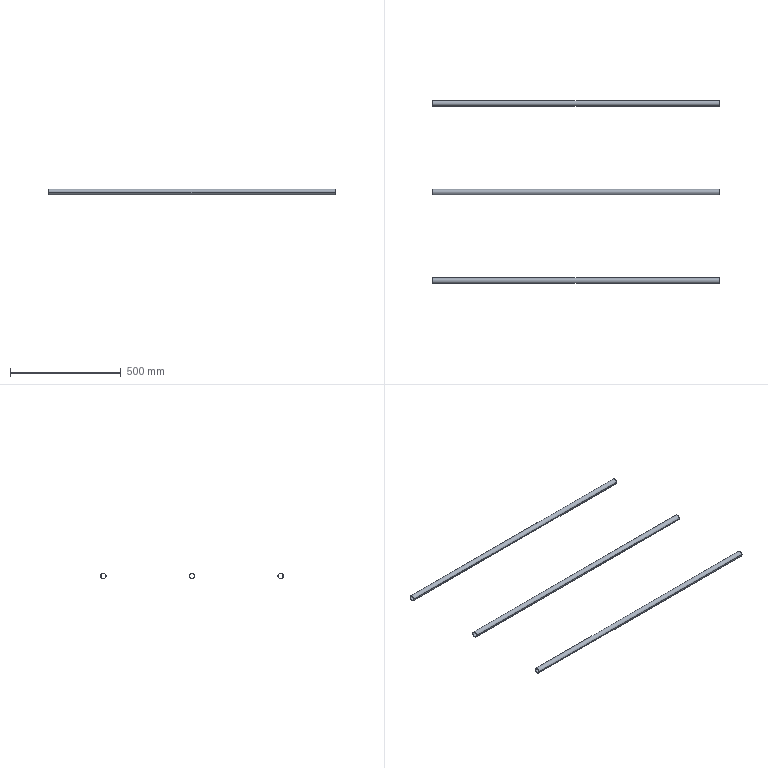Part | STEP file | E3-中转釜护栏6栏杆_Default<As Machined> | 3 solids | 18 faces | box 1295 x 825 x 25 mm | volume 430229 mm3 | cylinder 12 | plane 6 | commonest cylinder face diameters 22 x6 25 x6
STEP:
#1=CARTESIAN_POINT('',(0.,0.,0.));
#2=DIRECTION('',(0.,0.,1.));
#3=DIRECTION('',(1.,0.,0.));
#4=AXIS2_PLACEMENT_3D('',#1,#2,#3);
#5=CARTESIAN_POINT('',(647.5,787.5,0.));
#6=VERTEX_POINT('',#5);
#7=CARTESIAN_POINT('',(647.5,812.5,0.));
#8=VERTEX_POINT('',#7);
#9=CARTESIAN_POINT('',(647.5,800.,0.));
#10=DIRECTION('',(-1.,0.,0.));
#11=DIRECTION('',(0.,1.,0.));
#12=AXIS2_PLACEMENT_3D('',#9,#10,#11);
#13=CIRCLE('',#12,12.5);
#14=CARTESIAN_POINT('',(647.5,800.,0.));
#15=DIRECTION('',(-1.,0.,0.));
#16=DIRECTION('',(0.,-1.,0.));
#17=AXIS2_PLACEMENT_3D('',#14,#15,#16);
#18=CYLINDRICAL_SURFACE('',#17,12.5);
#19=CARTESIAN_POINT('',(-3.142,0.));
#20=DIRECTION('',(1.,0.));
#21=VECTOR('',#20,1.);
#22=LINE('',#19,#21);
#23=(GEOMETRIC_REPRESENTATION_CONTEXT(2)PARAMETRIC_REPRESENTATION_CONTEXT()REPRESENTATION_CONTEXT('',''));
#24=DEFINITIONAL_REPRESENTATION('',(#22),#23);
#25=PCURVE('',#18,#24);
#26=CARTESIAN_POINT('',(647.5,800.,0.));
#27=DIRECTION('',(1.,0.,0.));
#28=DIRECTION('',(0.,1.,0.));
#29=AXIS2_PLACEMENT_3D('',#26,#27,#28);
#30=PLANE('',#29);
#31=CARTESIAN_POINT('',(12.5,0.));
#32=CARTESIAN_POINT('',(12.5,-21.651));
#33=CARTESIAN_POINT('',(-6.25,-10.825));
#34=CARTESIAN_POINT('',(-25.,0.));
#35=CARTESIAN_POINT('',(-6.25,10.825));
#36=CARTESIAN_POINT('',(12.5,21.651));
#37=CARTESIAN_POINT('',(12.5,0.));
#38=(BOUNDED_CURVE()B_SPLINE_CURVE(2,(#31,#32,#33,#34,#35,#36,#37),.UNSPECIFIED.,.T.,.F.)B_SPLINE_CURVE_WITH_KNOTS((1,2,2,2,2,1),(-2.094,0.,2.094,4.189,6.283,8.378),.UNSPECIFIED.)CURVE()GEOMETRIC_REPRESENTATION_ITEM()RATIONAL_B_SPLINE_CURVE((1.,0.5,1.,0.5,1.,0.5,1.))REPRESENTATION_ITEM(''));
#39=(GEOMETRIC_REPRESENTATION_CONTEXT(2)PARAMETRIC_REPRESENTATION_CONTEXT()REPRESENTATION_CONTEXT('',''));
#40=DEFINITIONAL_REPRESENTATION('',(#38),#39);
#41=PCURVE('',#30,#40);
#42=SURFACE_CURVE('',#13,(#25,#41),.PCURVE_S1.);
#43=EDGE_CURVE('',#6,#8,#42,.T.);
#44=ORIENTED_EDGE('',*,*,#43,.T.);
#45=CARTESIAN_POINT('',(-647.5,812.5,0.));
#46=VERTEX_POINT('',#45);
#47=CARTESIAN_POINT('',(647.5,812.5,0.));
#48=DIRECTION('',(-1.,0.,0.));
#49=VECTOR('',#48,1.);
#50=LINE('',#47,#49);
#51=CARTESIAN_POINT('',(3.142,0.));
#52=DIRECTION('',(0.,1.));
#53=VECTOR('',#52,1.);
#54=LINE('',#51,#53);
#55=(GEOMETRIC_REPRESENTATION_CONTEXT(2)PARAMETRIC_REPRESENTATION_CONTEXT()REPRESENTATION_CONTEXT('',''));
#56=DEFINITIONAL_REPRESENTATION('',(#54),#55);
#57=PCURVE('',#18,#56);
#58=CARTESIAN_POINT('',(647.5,800.,0.));
#59=DIRECTION('',(-1.,0.,0.));
#60=DIRECTION('',(0.,-1.,0.));
#61=AXIS2_PLACEMENT_3D('',#58,#59,#60);
#62=CYLINDRICAL_SURFACE('',#61,12.5);
#63=CARTESIAN_POINT('',(3.142,0.));
#64=DIRECTION('',(0.,1.));
#65=VECTOR('',#64,1.);
#66=LINE('',#63,#65);
#67=(GEOMETRIC_REPRESENTATION_CONTEXT(2)PARAMETRIC_REPRESENTATION_CONTEXT()REPRESENTATION_CONTEXT('',''));
#68=DEFINITIONAL_REPRESENTATION('',(#66),#67);
#69=PCURVE('',#62,#68);
#70=SURFACE_CURVE('',#50,(#57,#69),.PCURVE_S1.);
#71=EDGE_CURVE('',#8,#46,#70,.T.);
#72=ORIENTED_EDGE('',*,*,#71,.T.);
#73=CARTESIAN_POINT('',(-647.5,787.5,0.));
#74=VERTEX_POINT('',#73);
#75=CARTESIAN_POINT('',(-647.5,800.,0.));
#76=DIRECTION('',(-1.,0.,0.));
#77=DIRECTION('',(0.,1.,0.));
#78=AXIS2_PLACEMENT_3D('',#75,#76,#77);
#79=CIRCLE('',#78,12.5);
#80=CARTESIAN_POINT('',(-3.142,1295.));
#81=DIRECTION('',(1.,0.));
#82=VECTOR('',#81,1.);
#83=LINE('',#80,#82);
#84=(GEOMETRIC_REPRESENTATION_CONTEXT(2)PARAMETRIC_REPRESENTATION_CONTEXT()REPRESENTATION_CONTEXT('',''));
#85=DEFINITIONAL_REPRESENTATION('',(#83),#84);
#86=PCURVE('',#18,#85);
#87=CARTESIAN_POINT('',(-647.5,800.,0.));
#88=DIRECTION('',(1.,0.,0.));
#89=DIRECTION('',(0.,1.,0.));
#90=AXIS2_PLACEMENT_3D('',#87,#88,#89);
#91=PLANE('',#90);
#92=CARTESIAN_POINT('',(12.5,0.));
#93=CARTESIAN_POINT('',(12.5,-21.651));
#94=CARTESIAN_POINT('',(-6.25,-10.825));
#95=CARTESIAN_POINT('',(-25.,0.));
#96=CARTESIAN_POINT('',(-6.25,10.825));
#97=CARTESIAN_POINT('',(12.5,21.651));
#98=CARTESIAN_POINT('',(12.5,0.));
#99=(BOUNDED_CURVE()B_SPLINE_CURVE(2,(#92,#93,#94,#95,#96,#97,#98),.UNSPECIFIED.,.T.,.F.)B_SPLINE_CURVE_WITH_KNOTS((1,2,2,2,2,1),(-2.094,0.,2.094,4.189,6.283,8.378),.UNSPECIFIED.)CURVE()GEOMETRIC_REPRESENTATION_ITEM()RATIONAL_B_SPLINE_CURVE((1.,0.5,1.,0.5,1.,0.5,1.))REPRESENTATION_ITEM(''));
#100=(GEOMETRIC_REPRESENTATION_CONTEXT(2)PARAMETRIC_REPRESENTATION_CONTEXT()REPRESENTATION_CONTEXT('',''));
#101=DEFINITIONAL_REPRESENTATION('',(#99),#100);
#102=PCURVE('',#91,#101);
#103=SURFACE_CURVE('',#79,(#86,#102),.PCURVE_S1.);
#104=EDGE_CURVE('',#74,#46,#103,.T.);
#105=ORIENTED_EDGE('',*,*,#104,.F.);
#106=CARTESIAN_POINT('',(647.5,787.5,0.));
#107=DIRECTION('',(-1.,0.,0.));
#108=VECTOR('',#107,1.);
#109=LINE('',#106,#108);
#110=CARTESIAN_POINT('',(0.,0.));
#111=DIRECTION('',(0.,1.));
#112=VECTOR('',#111,1.);
#113=LINE('',#110,#112);
#114=(GEOMETRIC_REPRESENTATION_CONTEXT(2)PARAMETRIC_REPRESENTATION_CONTEXT()REPRESENTATION_CONTEXT('',''));
#115=DEFINITIONAL_REPRESENTATION('',(#113),#114);
#116=PCURVE('',#18,#115);
#117=CARTESIAN_POINT('',(6.283,0.));
#118=DIRECTION('',(0.,1.));
#119=VECTOR('',#118,1.);
#120=LINE('',#117,#119);
#121=(GEOMETRIC_REPRESENTATION_CONTEXT(2)PARAMETRIC_REPRESENTATION_CONTEXT()REPRESENTATION_CONTEXT('',''));
#122=DEFINITIONAL_REPRESENTATION('',(#120),#121);
#123=PCURVE('',#62,#122);
#124=SURFACE_CURVE('',#109,(#116,#123),.PCURVE_S1.);
#125=EDGE_CURVE('',#6,#74,#124,.T.);
#126=ORIENTED_EDGE('',*,*,#125,.F.);
#127=EDGE_LOOP('',(#44,#72,#105,#126));
#128=FACE_BOUND('',#127,.T.);
#129=ADVANCED_FACE('',(#128),#18,.T.);
#130=CARTESIAN_POINT('',(647.5,789.,0.));
#131=VERTEX_POINT('',#130);
#132=CARTESIAN_POINT('',(-647.5,789.,0.));
#133=VERTEX_POINT('',#132);
#134=CARTESIAN_POINT('',(647.5,789.,0.));
#135=DIRECTION('',(-1.,0.,0.));
#136=VECTOR('',#135,1.);
#137=LINE('',#134,#136);
#138=CARTESIAN_POINT('',(647.5,800.,0.));
#139=DIRECTION('',(-1.,0.,0.));
#140=DIRECTION('',(0.,-1.,0.));
#141=AXIS2_PLACEMENT_3D('',#138,#139,#140);
#142=CYLINDRICAL_SURFACE('',#141,11.);
#143=CARTESIAN_POINT('',(6.283,0.));
#144=DIRECTION('',(0.,1.));
#145=VECTOR('',#144,1.);
#146=LINE('',#143,#145);
#147=(GEOMETRIC_REPRESENTATION_CONTEXT(2)PARAMETRIC_REPRESENTATION_CONTEXT()REPRESENTATION_CONTEXT('',''));
#148=DEFINITIONAL_REPRESENTATION('',(#146),#147);
#149=PCURVE('',#142,#148);
#150=CARTESIAN_POINT('',(647.5,800.,0.));
#151=DIRECTION('',(-1.,0.,0.));
#152=DIRECTION('',(0.,-1.,0.));
#153=AXIS2_PLACEMENT_3D('',#150,#151,#152);
#154=CYLINDRICAL_SURFACE('',#153,11.);
#155=CARTESIAN_POINT('',(0.,0.));
#156=DIRECTION('',(0.,1.));
#157=VECTOR('',#156,1.);
#158=LINE('',#155,#157);
#159=(GEOMETRIC_REPRESENTATION_CONTEXT(2)PARAMETRIC_REPRESENTATION_CONTEXT()REPRESENTATION_CONTEXT('',''));
#160=DEFINITIONAL_REPRESENTATION('',(#158),#159);
#161=PCURVE('',#154,#160);
#162=SURFACE_CURVE('',#137,(#149,#161),.PCURVE_S1.);
#163=EDGE_CURVE('',#131,#133,#162,.T.);
#164=ORIENTED_EDGE('',*,*,#163,.T.);
#165=CARTESIAN_POINT('',(-647.5,811.,0.));
#166=VERTEX_POINT('',#165);
#167=CARTESIAN_POINT('',(-647.5,800.,0.));
#168=DIRECTION('',(-1.,0.,0.));
#169=DIRECTION('',(0.,1.,0.));
#170=AXIS2_PLACEMENT_3D('',#167,#168,#169);
#171=CIRCLE('',#170,11.);
#172=CARTESIAN_POINT('',(3.142,1295.));
#173=DIRECTION('',(1.,0.));
#174=VECTOR('',#173,1.);
#175=LINE('',#172,#174);
#176=(GEOMETRIC_REPRESENTATION_CONTEXT(2)PARAMETRIC_REPRESENTATION_CONTEXT()REPRESENTATION_CONTEXT('',''));
#177=DEFINITIONAL_REPRESENTATION('',(#175),#176);
#178=PCURVE('',#142,#177);
#179=CARTESIAN_POINT('',(11.,0.));
#180=CARTESIAN_POINT('',(11.,-19.053));
#181=CARTESIAN_POINT('',(-5.5,-9.526));
#182=CARTESIAN_POINT('',(-22.,0.));
#183=CARTESIAN_POINT('',(-5.5,9.526));
#184=CARTESIAN_POINT('',(11.,19.053));
#185=CARTESIAN_POINT('',(11.,0.));
#186=(BOUNDED_CURVE()B_SPLINE_CURVE(2,(#179,#180,#181,#182,#183,#184,#185),.UNSPECIFIED.,.T.,.F.)B_SPLINE_CURVE_WITH_KNOTS((1,2,2,2,2,1),(-2.094,0.,2.094,4.189,6.283,8.378),.UNSPECIFIED.)CURVE()GEOMETRIC_REPRESENTATION_ITEM()RATIONAL_B_SPLINE_CURVE((1.,0.5,1.,0.5,1.,0.5,1.))REPRESENTATION_ITEM(''));
#187=(GEOMETRIC_REPRESENTATION_CONTEXT(2)PARAMETRIC_REPRESENTATION_CONTEXT()REPRESENTATION_CONTEXT('',''));
#188=DEFINITIONAL_REPRESENTATION('',(#186),#187);
#189=PCURVE('',#91,#188);
#190=SURFACE_CURVE('',#171,(#178,#189),.PCURVE_S1.);
#191=EDGE_CURVE('',#166,#133,#190,.T.);
#192=ORIENTED_EDGE('',*,*,#191,.F.);
#193=CARTESIAN_POINT('',(647.5,811.,0.));
#194=VERTEX_POINT('',#193);
#195=CARTESIAN_POINT('',(647.5,811.,0.));
#196=DIRECTION('',(-1.,0.,0.));
#197=VECTOR('',#196,1.);
#198=LINE('',#195,#197);
#199=CARTESIAN_POINT('',(3.142,0.));
#200=DIRECTION('',(0.,1.));
#201=VECTOR('',#200,1.);
#202=LINE('',#199,#201);
#203=(GEOMETRIC_REPRESENTATION_CONTEXT(2)PARAMETRIC_REPRESENTATION_CONTEXT()REPRESENTATION_CONTEXT('',''));
#204=DEFINITIONAL_REPRESENTATION('',(#202),#203);
#205=PCURVE('',#142,#204);
#206=CARTESIAN_POINT('',(3.142,0.));
#207=DIRECTION('',(0.,1.));
#208=VECTOR('',#207,1.);
#209=LINE('',#206,#208);
#210=(GEOMETRIC_REPRESENTATION_CONTEXT(2)PARAMETRIC_REPRESENTATION_CONTEXT()REPRESENTATION_CONTEXT('',''));
#211=DEFINITIONAL_REPRESENTATION('',(#209),#210);
#212=PCURVE('',#154,#211);
#213=SURFACE_CURVE('',#198,(#205,#212),.PCURVE_S1.);
#214=EDGE_CURVE('',#194,#166,#213,.T.);
#215=ORIENTED_EDGE('',*,*,#214,.F.);
#216=CARTESIAN_POINT('',(647.5,800.,0.));
#217=DIRECTION('',(-1.,0.,0.));
#218=DIRECTION('',(0.,1.,0.));
#219=AXIS2_PLACEMENT_3D('',#216,#217,#218);
#220=CIRCLE('',#219,11.);
#221=CARTESIAN_POINT('',(3.142,0.));
#222=DIRECTION('',(1.,0.));
#223=VECTOR('',#222,1.);
#224=LINE('',#221,#223);
#225=(GEOMETRIC_REPRESENTATION_CONTEXT(2)PARAMETRIC_REPRESENTATION_CONTEXT()REPRESENTATION_CONTEXT('',''));
#226=DEFINITIONAL_REPRESENTATION('',(#224),#225);
#227=PCURVE('',#142,#226);
#228=CARTESIAN_POINT('',(11.,0.));
#229=CARTESIAN_POINT('',(11.,-19.053));
#230=CARTESIAN_POINT('',(-5.5,-9.526));
#231=CARTESIAN_POINT('',(-22.,0.));
#232=CARTESIAN_POINT('',(-5.5,9.526));
#233=CARTESIAN_POINT('',(11.,19.053));
#234=CARTESIAN_POINT('',(11.,0.));
#235=(BOUNDED_CURVE()B_SPLINE_CURVE(2,(#228,#229,#230,#231,#232,#233,#234),.UNSPECIFIED.,.T.,.F.)B_SPLINE_CURVE_WITH_KNOTS((1,2,2,2,2,1),(-2.094,0.,2.094,4.189,6.283,8.378),.UNSPECIFIED.)CURVE()GEOMETRIC_REPRESENTATION_ITEM()RATIONAL_B_SPLINE_CURVE((1.,0.5,1.,0.5,1.,0.5,1.))REPRESENTATION_ITEM(''));
#236=(GEOMETRIC_REPRESENTATION_CONTEXT(2)PARAMETRIC_REPRESENTATION_CONTEXT()REPRESENTATION_CONTEXT('',''));
#237=DEFINITIONAL_REPRESENTATION('',(#235),#236);
#238=PCURVE('',#30,#237);
#239=SURFACE_CURVE('',#220,(#227,#238),.PCURVE_S1.);
#240=EDGE_CURVE('',#194,#131,#239,.T.);
#241=ORIENTED_EDGE('',*,*,#240,.T.);
#242=EDGE_LOOP('',(#164,#192,#215,#241));
#243=FACE_BOUND('',#242,.F.);
#244=ADVANCED_FACE('',(#243),#142,.F.);
#245=CARTESIAN_POINT('',(-647.5,800.,0.));
#246=DIRECTION('',(-1.,0.,0.));
#247=DIRECTION('',(0.,1.,0.));
#248=AXIS2_PLACEMENT_3D('',#245,#246,#247);
#249=CIRCLE('',#248,11.);
#250=CARTESIAN_POINT('',(-3.142,1295.));
#251=DIRECTION('',(1.,0.));
#252=VECTOR('',#251,1.);
#253=LINE('',#250,#252);
#254=(GEOMETRIC_REPRESENTATION_CONTEXT(2)PARAMETRIC_REPRESENTATION_CONTEXT()REPRESENTATION_CONTEXT('',''));
#255=DEFINITIONAL_REPRESENTATION('',(#253),#254);
#256=PCURVE('',#154,#255);
#257=CARTESIAN_POINT('',(11.,0.));
#258=CARTESIAN_POINT('',(11.,-19.053));
#259=CARTESIAN_POINT('',(-5.5,-9.526));
#260=CARTESIAN_POINT('',(-22.,0.));
#261=CARTESIAN_POINT('',(-5.5,9.526));
#262=CARTESIAN_POINT('',(11.,19.053));
#263=CARTESIAN_POINT('',(11.,0.));
#264=(BOUNDED_CURVE()B_SPLINE_CURVE(2,(#257,#258,#259,#260,#261,#262,#263),.UNSPECIFIED.,.T.,.F.)B_SPLINE_CURVE_WITH_KNOTS((1,2,2,2,2,1),(-2.094,0.,2.094,4.189,6.283,8.378),.UNSPECIFIED.)CURVE()GEOMETRIC_REPRESENTATION_ITEM()RATIONAL_B_SPLINE_CURVE((1.,0.5,1.,0.5,1.,0.5,1.))REPRESENTATION_ITEM(''));
#265=(GEOMETRIC_REPRESENTATION_CONTEXT(2)PARAMETRIC_REPRESENTATION_CONTEXT()REPRESENTATION_CONTEXT('',''));
#266=DEFINITIONAL_REPRESENTATION('',(#264),#265);
#267=PCURVE('',#91,#266);
#268=SURFACE_CURVE('',#249,(#256,#267),.PCURVE_S1.);
#269=EDGE_CURVE('',#133,#166,#268,.T.);
#270=ORIENTED_EDGE('',*,*,#269,.F.);
#271=ORIENTED_EDGE('',*,*,#163,.F.);
#272=CARTESIAN_POINT('',(647.5,800.,0.));
#273=DIRECTION('',(-1.,0.,0.));
#274=DIRECTION('',(0.,1.,0.));
#275=AXIS2_PLACEMENT_3D('',#272,#273,#274);
#276=CIRCLE('',#275,11.);
#277=CARTESIAN_POINT('',(-3.142,0.));
#278=DIRECTION('',(1.,0.));
#279=VECTOR('',#278,1.);
#280=LINE('',#277,#279);
#281=(GEOMETRIC_REPRESENTATION_CONTEXT(2)PARAMETRIC_REPRESENTATION_CONTEXT()REPRESENTATION_CONTEXT('',''));
#282=DEFINITIONAL_REPRESENTATION('',(#280),#281);
#283=PCURVE('',#154,#282);
#284=CARTESIAN_POINT('',(11.,0.));
#285=CARTESIAN_POINT('',(11.,-19.053));
#286=CARTESIAN_POINT('',(-5.5,-9.526));
#287=CARTESIAN_POINT('',(-22.,0.));
#288=CARTESIAN_POINT('',(-5.5,9.526));
#289=CARTESIAN_POINT('',(11.,19.053));
#290=CARTESIAN_POINT('',(11.,0.));
#291=(BOUNDED_CURVE()B_SPLINE_CURVE(2,(#284,#285,#286,#287,#288,#289,#290),.UNSPECIFIED.,.T.,.F.)B_SPLINE_CURVE_WITH_KNOTS((1,2,2,2,2,1),(-2.094,0.,2.094,4.189,6.283,8.378),.UNSPECIFIED.)CURVE()GEOMETRIC_REPRESENTATION_ITEM()RATIONAL_B_SPLINE_CURVE((1.,0.5,1.,0.5,1.,0.5,1.))REPRESENTATION_ITEM(''));
#292=(GEOMETRIC_REPRESENTATION_CONTEXT(2)PARAMETRIC_REPRESENTATION_CONTEXT()REPRESENTATION_CONTEXT('',''));
#293=DEFINITIONAL_REPRESENTATION('',(#291),#292);
#294=PCURVE('',#30,#293);
#295=SURFACE_CURVE('',#276,(#283,#294),.PCURVE_S1.);
#296=EDGE_CURVE('',#131,#194,#295,.T.);
#297=ORIENTED_EDGE('',*,*,#296,.T.);
#298=ORIENTED_EDGE('',*,*,#214,.T.);
#299=EDGE_LOOP('',(#270,#271,#297,#298));
#300=FACE_BOUND('',#299,.F.);
#301=ADVANCED_FACE('',(#300),#154,.F.);
#302=ORIENTED_EDGE('',*,*,#71,.F.);
#303=CARTESIAN_POINT('',(647.5,800.,0.));
#304=DIRECTION('',(-1.,0.,0.));
#305=DIRECTION('',(0.,1.,0.));
#306=AXIS2_PLACEMENT_3D('',#303,#304,#305);
#307=CIRCLE('',#306,12.5);
#308=CARTESIAN_POINT('',(3.142,0.));
#309=DIRECTION('',(1.,0.));
#310=VECTOR('',#309,1.);
#311=LINE('',#308,#310);
#312=(GEOMETRIC_REPRESENTATION_CONTEXT(2)PARAMETRIC_REPRESENTATION_CONTEXT()REPRESENTATION_CONTEXT('',''));
#313=DEFINITIONAL_REPRESENTATION('',(#311),#312);
#314=PCURVE('',#62,#313);
#315=CARTESIAN_POINT('',(12.5,0.));
#316=CARTESIAN_POINT('',(12.5,-21.651));
#317=CARTESIAN_POINT('',(-6.25,-10.825));
#318=CARTESIAN_POINT('',(-25.,0.));
#319=CARTESIAN_POINT('',(-6.25,10.825));
#320=CARTESIAN_POINT('',(12.5,21.651));
#321=CARTESIAN_POINT('',(12.5,0.));
#322=(BOUNDED_CURVE()B_SPLINE_CURVE(2,(#315,#316,#317,#318,#319,#320,#321),.UNSPECIFIED.,.T.,.F.)B_SPLINE_CURVE_WITH_KNOTS((1,2,2,2,2,1),(-2.094,0.,2.094,4.189,6.283,8.378),.UNSPECIFIED.)CURVE()GEOMETRIC_REPRESENTATION_ITEM()RATIONAL_B_SPLINE_CURVE((1.,0.5,1.,0.5,1.,0.5,1.))REPRESENTATION_ITEM(''));
#323=(GEOMETRIC_REPRESENTATION_CONTEXT(2)PARAMETRIC_REPRESENTATION_CONTEXT()REPRESENTATION_CONTEXT('',''));
#324=DEFINITIONAL_REPRESENTATION('',(#322),#323);
#325=PCURVE('',#30,#324);
#326=SURFACE_CURVE('',#307,(#314,#325),.PCURVE_S1.);
#327=EDGE_CURVE('',#8,#6,#326,.T.);
#328=ORIENTED_EDGE('',*,*,#327,.T.);
#329=ORIENTED_EDGE('',*,*,#125,.T.);
#330=CARTESIAN_POINT('',(-647.5,800.,0.));
#331=DIRECTION('',(-1.,0.,0.));
#332=DIRECTION('',(0.,1.,0.));
#333=AXIS2_PLACEMENT_3D('',#330,#331,#332);
#334=CIRCLE('',#333,12.5);
#335=CARTESIAN_POINT('',(3.142,1295.));
#336=DIRECTION('',(1.,0.));
#337=VECTOR('',#336,1.);
#338=LINE('',#335,#337);
#339=(GEOMETRIC_REPRESENTATION_CONTEXT(2)PARAMETRIC_REPRESENTATION_CONTEXT()REPRESENTATION_CONTEXT('',''));
#340=DEFINITIONAL_REPRESENTATION('',(#338),#339);
#341=PCURVE('',#62,#340);
#342=CARTESIAN_POINT('',(12.5,0.));
#343=CARTESIAN_POINT('',(12.5,-21.651));
#344=CARTESIAN_POINT('',(-6.25,-10.825));
#345=CARTESIAN_POINT('',(-25.,0.));
#346=CARTESIAN_POINT('',(-6.25,10.825));
#347=CARTESIAN_POINT('',(12.5,21.651));
#348=CARTESIAN_POINT('',(12.5,0.));
#349=(BOUNDED_CURVE()B_SPLINE_CURVE(2,(#342,#343,#344,#345,#346,#347,#348),.UNSPECIFIED.,.T.,.F.)B_SPLINE_CURVE_WITH_KNOTS((1,2,2,2,2,1),(-2.094,0.,2.094,4.189,6.283,8.378),.UNSPECIFIED.)CURVE()GEOMETRIC_REPRESENTATION_ITEM()RATIONAL_B_SPLINE_CURVE((1.,0.5,1.,0.5,1.,0.5,1.))REPRESENTATION_ITEM(''));
#350=(GEOMETRIC_REPRESENTATION_CONTEXT(2)PARAMETRIC_REPRESENTATION_CONTEXT()REPRESENTATION_CONTEXT('',''));
#351=DEFINITIONAL_REPRESENTATION('',(#349),#350);
#352=PCURVE('',#91,#351);
#353=SURFACE_CURVE('',#334,(#341,#352),.PCURVE_S1.);
#354=EDGE_CURVE('',#46,#74,#353,.T.);
#355=ORIENTED_EDGE('',*,*,#354,.F.);
#356=EDGE_LOOP('',(#302,#328,#329,#355));
#357=FACE_BOUND('',#356,.T.);
#358=ADVANCED_FACE('',(#357),#62,.T.);
#359=ORIENTED_EDGE('',*,*,#296,.T.);
#360=ORIENTED_EDGE('',*,*,#240,.T.);
#361=EDGE_LOOP('',(#359,#360));
#362=FACE_BOUND('',#361,.T.);
#363=ORIENTED_EDGE('',*,*,#43,.F.);
#364=ORIENTED_EDGE('',*,*,#327,.F.);
#365=EDGE_LOOP('',(#363,#364));
#366=FACE_BOUND('',#365,.T.);
#367=ADVANCED_FACE('',(#362,#366),#30,.T.);
#368=ORIENTED_EDGE('',*,*,#269,.F.);
#369=ORIENTED_EDGE('',*,*,#191,.F.);
#370=EDGE_LOOP('',(#368,#369));
#371=FACE_BOUND('',#370,.T.);
#372=ORIENTED_EDGE('',*,*,#104,.T.);
#373=ORIENTED_EDGE('',*,*,#354,.T.);
#374=EDGE_LOOP('',(#372,#373));
#375=FACE_BOUND('',#374,.T.);
#376=ADVANCED_FACE('',(#371,#375),#91,.F.);
#377=CLOSED_SHELL('',(#129,#244,#301,#358,#367,#376));
#378=MANIFOLD_SOLID_BREP('',#377);
#379=CARTESIAN_POINT('',(647.5,-12.5,0.));
#380=VERTEX_POINT('',#379);
#381=CARTESIAN_POINT('',(647.5,12.5,0.));
#382=VERTEX_POINT('',#381);
#383=CARTESIAN_POINT('',(647.5,0.,0.));
#384=DIRECTION('',(-1.,0.,0.));
#385=DIRECTION('',(0.,1.,0.));
#386=AXIS2_PLACEMENT_3D('',#383,#384,#385);
#387=CIRCLE('',#386,12.5);
#388=CARTESIAN_POINT('',(647.5,0.,0.));
#389=DIRECTION('',(-1.,0.,0.));
#390=DIRECTION('',(0.,-1.,0.));
#391=AXIS2_PLACEMENT_3D('',#388,#389,#390);
#392=CYLINDRICAL_SURFACE('',#391,12.5);
#393=CARTESIAN_POINT('',(-3.142,0.));
#394=DIRECTION('',(1.,0.));
#395=VECTOR('',#394,1.);
#396=LINE('',#393,#395);
#397=(GEOMETRIC_REPRESENTATION_CONTEXT(2)PARAMETRIC_REPRESENTATION_CONTEXT()REPRESENTATION_CONTEXT('',''));
#398=DEFINITIONAL_REPRESENTATION('',(#396),#397);
#399=PCURVE('',#392,#398);
#400=CARTESIAN_POINT('',(647.5,0.,0.));
#401=DIRECTION('',(1.,0.,0.));
#402=DIRECTION('',(0.,1.,0.));
#403=AXIS2_PLACEMENT_3D('',#400,#401,#402);
#404=PLANE('',#403);
#405=CARTESIAN_POINT('',(12.5,0.));
#406=CARTESIAN_POINT('',(12.5,-21.651));
#407=CARTESIAN_POINT('',(-6.25,-10.825));
#408=CARTESIAN_POINT('',(-25.,0.));
#409=CARTESIAN_POINT('',(-6.25,10.825));
#410=CARTESIAN_POINT('',(12.5,21.651));
#411=CARTESIAN_POINT('',(12.5,0.));
#412=(BOUNDED_CURVE()B_SPLINE_CURVE(2,(#405,#406,#407,#408,#409,#410,#411),.UNSPECIFIED.,.T.,.F.)B_SPLINE_CURVE_WITH_KNOTS((1,2,2,2,2,1),(-2.094,0.,2.094,4.189,6.283,8.378),.UNSPECIFIED.)CURVE()GEOMETRIC_REPRESENTATION_ITEM()RATIONAL_B_SPLINE_CURVE((1.,0.5,1.,0.5,1.,0.5,1.))REPRESENTATION_ITEM(''));
#413=(GEOMETRIC_REPRESENTATION_CONTEXT(2)PARAMETRIC_REPRESENTATION_CONTEXT()REPRESENTATION_CONTEXT('',''));
#414=DEFINITIONAL_REPRESENTATION('',(#412),#413);
#415=PCURVE('',#404,#414);
#416=SURFACE_CURVE('',#387,(#399,#415),.PCURVE_S1.);
#417=EDGE_CURVE('',#380,#382,#416,.T.);
#418=ORIENTED_EDGE('',*,*,#417,.T.);
#419=CARTESIAN_POINT('',(-647.5,12.5,0.));
#420=VERTEX_POINT('',#419);
#421=CARTESIAN_POINT('',(647.5,12.5,0.));
#422=DIRECTION('',(-1.,0.,0.));
#423=VECTOR('',#422,1.);
#424=LINE('',#421,#423);
#425=CARTESIAN_POINT('',(3.142,0.));
#426=DIRECTION('',(0.,1.));
#427=VECTOR('',#426,1.);
#428=LINE('',#425,#427);
#429=(GEOMETRIC_REPRESENTATION_CONTEXT(2)PARAMETRIC_REPRESENTATION_CONTEXT()REPRESENTATION_CONTEXT('',''));
#430=DEFINITIONAL_REPRESENTATION('',(#428),#429);
#431=PCURVE('',#392,#430);
#432=CARTESIAN_POINT('',(647.5,0.,0.));
#433=DIRECTION('',(-1.,0.,0.));
#434=DIRECTION('',(0.,-1.,0.));
#435=AXIS2_PLACEMENT_3D('',#432,#433,#434);
#436=CYLINDRICAL_SURFACE('',#435,12.5);
#437=CARTESIAN_POINT('',(3.142,0.));
#438=DIRECTION('',(0.,1.));
#439=VECTOR('',#438,1.);
#440=LINE('',#437,#439);
#441=(GEOMETRIC_REPRESENTATION_CONTEXT(2)PARAMETRIC_REPRESENTATION_CONTEXT()REPRESENTATION_CONTEXT('',''));
#442=DEFINITIONAL_REPRESENTATION('',(#440),#441);
#443=PCURVE('',#436,#442);
#444=SURFACE_CURVE('',#424,(#431,#443),.PCURVE_S1.);
#445=EDGE_CURVE('',#382,#420,#444,.T.);
#446=ORIENTED_EDGE('',*,*,#445,.T.);
#447=CARTESIAN_POINT('',(-647.5,-12.5,0.));
#448=VERTEX_POINT('',#447);
#449=CARTESIAN_POINT('',(-647.5,0.,0.));
#450=DIRECTION('',(-1.,0.,0.));
#451=DIRECTION('',(0.,1.,0.));
#452=AXIS2_PLACEMENT_3D('',#449,#450,#451);
#453=CIRCLE('',#452,12.5);
#454=CARTESIAN_POINT('',(-3.142,1295.));
#455=DIRECTION('',(1.,0.));
#456=VECTOR('',#455,1.);
#457=LINE('',#454,#456);
#458=(GEOMETRIC_REPRESENTATION_CONTEXT(2)PARAMETRIC_REPRESENTATION_CONTEXT()REPRESENTATION_CONTEXT('',''));
#459=DEFINITIONAL_REPRESENTATION('',(#457),#458);
#460=PCURVE('',#392,#459);
#461=CARTESIAN_POINT('',(-647.5,0.,0.));
#462=DIRECTION('',(1.,0.,0.));
#463=DIRECTION('',(0.,1.,0.));
#464=AXIS2_PLACEMENT_3D('',#461,#462,#463);
#465=PLANE('',#464);
#466=CARTESIAN_POINT('',(12.5,0.));
#467=CARTESIAN_POINT('',(12.5,-21.651));
#468=CARTESIAN_POINT('',(-6.25,-10.825));
#469=CARTESIAN_POINT('',(-25.,0.));
#470=CARTESIAN_POINT('',(-6.25,10.825));
#471=CARTESIAN_POINT('',(12.5,21.651));
#472=CARTESIAN_POINT('',(12.5,0.));
#473=(BOUNDED_CURVE()B_SPLINE_CURVE(2,(#466,#467,#468,#469,#470,#471,#472),.UNSPECIFIED.,.T.,.F.)B_SPLINE_CURVE_WITH_KNOTS((1,2,2,2,2,1),(-2.094,0.,2.094,4.189,6.283,8.378),.UNSPECIFIED.)CURVE()GEOMETRIC_REPRESENTATION_ITEM()RATIONAL_B_SPLINE_CURVE((1.,0.5,1.,0.5,1.,0.5,1.))REPRESENTATION_ITEM(''));
#474=(GEOMETRIC_REPRESENTATION_CONTEXT(2)PARAMETRIC_REPRESENTATION_CONTEXT()REPRESENTATION_CONTEXT('',''));
#475=DEFINITIONAL_REPRESENTATION('',(#473),#474);
#476=PCURVE('',#465,#475);
#477=SURFACE_CURVE('',#453,(#460,#476),.PCURVE_S1.);
#478=EDGE_CURVE('',#448,#420,#477,.T.);
#479=ORIENTED_EDGE('',*,*,#478,.F.);
#480=CARTESIAN_POINT('',(647.5,-12.5,0.));
#481=DIRECTION('',(-1.,0.,0.));
#482=VECTOR('',#481,1.);
#483=LINE('',#480,#482);
#484=CARTESIAN_POINT('',(0.,0.));
#485=DIRECTION('',(0.,1.));
#486=VECTOR('',#485,1.);
#487=LINE('',#484,#486);
#488=(GEOMETRIC_REPRESENTATION_CONTEXT(2)PARAMETRIC_REPRESENTATION_CONTEXT()REPRESENTATION_CONTEXT('',''));
#489=DEFINITIONAL_REPRESENTATION('',(#487),#488);
#490=PCURVE('',#392,#489);
#491=CARTESIAN_POINT('',(6.283,0.));
#492=DIRECTION('',(0.,1.));
#493=VECTOR('',#492,1.);
#494=LINE('',#491,#493);
#495=(GEOMETRIC_REPRESENTATION_CONTEXT(2)PARAMETRIC_REPRESENTATION_CONTEXT()REPRESENTATION_CONTEXT('',''));
#496=DEFINITIONAL_REPRESENTATION('',(#494),#495);
#497=PCURVE('',#436,#496);
#498=SURFACE_CURVE('',#483,(#490,#497),.PCURVE_S1.);
#499=EDGE_CURVE('',#380,#448,#498,.T.);
#500=ORIENTED_EDGE('',*,*,#499,.F.);
#501=EDGE_LOOP('',(#418,#446,#479,#500));
#502=FACE_BOUND('',#501,.T.);
#503=ADVANCED_FACE('',(#502),#392,.T.);
#504=CARTESIAN_POINT('',(647.5,-11.,0.));
#505=VERTEX_POINT('',#504);
#506=CARTESIAN_POINT('',(-647.5,-11.,0.));
#507=VERTEX_POINT('',#506);
#508=CARTESIAN_POINT('',(647.5,-11.,0.));
#509=DIRECTION('',(-1.,0.,0.));
#510=VECTOR('',#509,1.);
#511=LINE('',#508,#510);
#512=CARTESIAN_POINT('',(647.5,0.,0.));
#513=DIRECTION('',(-1.,0.,0.));
#514=DIRECTION('',(0.,-1.,0.));
#515=AXIS2_PLACEMENT_3D('',#512,#513,#514);
#516=CYLINDRICAL_SURFACE('',#515,11.);
#517=CARTESIAN_POINT('',(6.283,0.));
#518=DIRECTION('',(0.,1.));
#519=VECTOR('',#518,1.);
#520=LINE('',#517,#519);
#521=(GEOMETRIC_REPRESENTATION_CONTEXT(2)PARAMETRIC_REPRESENTATION_CONTEXT()REPRESENTATION_CONTEXT('',''));
#522=DEFINITIONAL_REPRESENTATION('',(#520),#521);
#523=PCURVE('',#516,#522);
#524=CARTESIAN_POINT('',(647.5,0.,0.));
#525=DIRECTION('',(-1.,0.,0.));
#526=DIRECTION('',(0.,-1.,0.));
#527=AXIS2_PLACEMENT_3D('',#524,#525,#526);
#528=CYLINDRICAL_SURFACE('',#527,11.);
#529=CARTESIAN_POINT('',(0.,0.));
#530=DIRECTION('',(0.,1.));
#531=VECTOR('',#530,1.);
#532=LINE('',#529,#531);
#533=(GEOMETRIC_REPRESENTATION_CONTEXT(2)PARAMETRIC_REPRESENTATION_CONTEXT()REPRESENTATION_CONTEXT('',''));
#534=DEFINITIONAL_REPRESENTATION('',(#532),#533);
#535=PCURVE('',#528,#534);
#536=SURFACE_CURVE('',#511,(#523,#535),.PCURVE_S1.);
#537=EDGE_CURVE('',#505,#507,#536,.T.);
#538=ORIENTED_EDGE('',*,*,#537,.T.);
#539=CARTESIAN_POINT('',(-647.5,11.,0.));
#540=VERTEX_POINT('',#539);
#541=CARTESIAN_POINT('',(-647.5,0.,0.));
#542=DIRECTION('',(-1.,0.,0.));
#543=DIRECTION('',(0.,1.,0.));
#544=AXIS2_PLACEMENT_3D('',#541,#542,#543);
#545=CIRCLE('',#544,11.);
#546=CARTESIAN_POINT('',(3.142,1295.));
#547=DIRECTION('',(1.,0.));
#548=VECTOR('',#547,1.);
#549=LINE('',#546,#548);
#550=(GEOMETRIC_REPRESENTATION_CONTEXT(2)PARAMETRIC_REPRESENTATION_CONTEXT()REPRESENTATION_CONTEXT('',''));
#551=DEFINITIONAL_REPRESENTATION('',(#549),#550);
#552=PCURVE('',#516,#551);
#553=CARTESIAN_POINT('',(11.,0.));
#554=CARTESIAN_POINT('',(11.,-19.053));
#555=CARTESIAN_POINT('',(-5.5,-9.526));
#556=CARTESIAN_POINT('',(-22.,0.));
#557=CARTESIAN_POINT('',(-5.5,9.526));
#558=CARTESIAN_POINT('',(11.,19.053));
#559=CARTESIAN_POINT('',(11.,0.));
#560=(BOUNDED_CURVE()B_SPLINE_CURVE(2,(#553,#554,#555,#556,#557,#558,#559),.UNSPECIFIED.,.T.,.F.)B_SPLINE_CURVE_WITH_KNOTS((1,2,2,2,2,1),(-2.094,0.,2.094,4.189,6.283,8.378),.UNSPECIFIED.)CURVE()GEOMETRIC_REPRESENTATION_ITEM()RATIONAL_B_SPLINE_CURVE((1.,0.5,1.,0.5,1.,0.5,1.))REPRESENTATION_ITEM(''));
#561=(GEOMETRIC_REPRESENTATION_CONTEXT(2)PARAMETRIC_REPRESENTATION_CONTEXT()REPRESENTATION_CONTEXT('',''));
#562=DEFINITIONAL_REPRESENTATION('',(#560),#561);
#563=PCURVE('',#465,#562);
#564=SURFACE_CURVE('',#545,(#552,#563),.PCURVE_S1.);
#565=EDGE_CURVE('',#540,#507,#564,.T.);
#566=ORIENTED_EDGE('',*,*,#565,.F.);
#567=CARTESIAN_POINT('',(647.5,11.,0.));
#568=VERTEX_POINT('',#567);
#569=CARTESIAN_POINT('',(647.5,11.,0.));
#570=DIRECTION('',(-1.,0.,0.));
#571=VECTOR('',#570,1.);
#572=LINE('',#569,#571);
#573=CARTESIAN_POINT('',(3.142,0.));
#574=DIRECTION('',(0.,1.));
#575=VECTOR('',#574,1.);
#576=LINE('',#573,#575);
#577=(GEOMETRIC_REPRESENTATION_CONTEXT(2)PARAMETRIC_REPRESENTATION_CONTEXT()REPRESENTATION_CONTEXT('',''));
#578=DEFINITIONAL_REPRESENTATION('',(#576),#577);
#579=PCURVE('',#516,#578);
#580=CARTESIAN_POINT('',(3.142,0.));
#581=DIRECTION('',(0.,1.));
#582=VECTOR('',#581,1.);
#583=LINE('',#580,#582);
#584=(GEOMETRIC_REPRESENTATION_CONTEXT(2)PARAMETRIC_REPRESENTATION_CONTEXT()REPRESENTATION_CONTEXT('',''));
#585=DEFINITIONAL_REPRESENTATION('',(#583),#584);
#586=PCURVE('',#528,#585);
#587=SURFACE_CURVE('',#572,(#579,#586),.PCURVE_S1.);
#588=EDGE_CURVE('',#568,#540,#587,.T.);
#589=ORIENTED_EDGE('',*,*,#588,.F.);
#590=CARTESIAN_POINT('',(647.5,0.,0.));
#591=DIRECTION('',(-1.,0.,0.));
#592=DIRECTION('',(0.,1.,0.));
#593=AXIS2_PLACEMENT_3D('',#590,#591,#592);
#594=CIRCLE('',#593,11.);
#595=CARTESIAN_POINT('',(3.142,0.));
#596=DIRECTION('',(1.,0.));
#597=VECTOR('',#596,1.);
#598=LINE('',#595,#597);
#599=(GEOMETRIC_REPRESENTATION_CONTEXT(2)PARAMETRIC_REPRESENTATION_CONTEXT()REPRESENTATION_CONTEXT('',''));
#600=DEFINITIONAL_REPRESENTATION('',(#598),#599);
#601=PCURVE('',#516,#600);
#602=CARTESIAN_POINT('',(11.,0.));
#603=CARTESIAN_POINT('',(11.,-19.053));
#604=CARTESIAN_POINT('',(-5.5,-9.526));
#605=CARTESIAN_POINT('',(-22.,0.));
#606=CARTESIAN_POINT('',(-5.5,9.526));
#607=CARTESIAN_POINT('',(11.,19.053));
#608=CARTESIAN_POINT('',(11.,0.));
#609=(BOUNDED_CURVE()B_SPLINE_CURVE(2,(#602,#603,#604,#605,#606,#607,#608),.UNSPECIFIED.,.T.,.F.)B_SPLINE_CURVE_WITH_KNOTS((1,2,2,2,2,1),(-2.094,0.,2.094,4.189,6.283,8.378),.UNSPECIFIED.)CURVE()GEOMETRIC_REPRESENTATION_ITEM()RATIONAL_B_SPLINE_CURVE((1.,0.5,1.,0.5,1.,0.5,1.))REPRESENTATION_ITEM(''));
#610=(GEOMETRIC_REPRESENTATION_CONTEXT(2)PARAMETRIC_REPRESENTATION_CONTEXT()REPRESENTATION_CONTEXT('',''));
#611=DEFINITIONAL_REPRESENTATION('',(#609),#610);
#612=PCURVE('',#404,#611);
#613=SURFACE_CURVE('',#594,(#601,#612),.PCURVE_S1.);
#614=EDGE_CURVE('',#568,#505,#613,.T.);
#615=ORIENTED_EDGE('',*,*,#614,.T.);
#616=EDGE_LOOP('',(#538,#566,#589,#615));
#617=FACE_BOUND('',#616,.F.);
#618=ADVANCED_FACE('',(#617),#516,.F.);
#619=CARTESIAN_POINT('',(-647.5,0.,0.));
#620=DIRECTION('',(-1.,0.,0.));
#621=DIRECTION('',(0.,1.,0.));
#622=AXIS2_PLACEMENT_3D('',#619,#620,#621);
#623=CIRCLE('',#622,11.);
#624=CARTESIAN_POINT('',(-3.142,1295.));
#625=DIRECTION('',(1.,0.));
#626=VECTOR('',#625,1.);
#627=LINE('',#624,#626);
#628=(GEOMETRIC_REPRESENTATION_CONTEXT(2)PARAMETRIC_REPRESENTATION_CONTEXT()REPRESENTATION_CONTEXT('',''));
#629=DEFINITIONAL_REPRESENTATION('',(#627),#628);
#630=PCURVE('',#528,#629);
#631=CARTESIAN_POINT('',(11.,0.));
#632=CARTESIAN_POINT('',(11.,-19.053));
#633=CARTESIAN_POINT('',(-5.5,-9.526));
#634=CARTESIAN_POINT('',(-22.,0.));
#635=CARTESIAN_POINT('',(-5.5,9.526));
#636=CARTESIAN_POINT('',(11.,19.053));
#637=CARTESIAN_POINT('',(11.,0.));
#638=(BOUNDED_CURVE()B_SPLINE_CURVE(2,(#631,#632,#633,#634,#635,#636,#637),.UNSPECIFIED.,.T.,.F.)B_SPLINE_CURVE_WITH_KNOTS((1,2,2,2,2,1),(-2.094,0.,2.094,4.189,6.283,8.378),.UNSPECIFIED.)CURVE()GEOMETRIC_REPRESENTATION_ITEM()RATIONAL_B_SPLINE_CURVE((1.,0.5,1.,0.5,1.,0.5,1.))REPRESENTATION_ITEM(''));
#639=(GEOMETRIC_REPRESENTATION_CONTEXT(2)PARAMETRIC_REPRESENTATION_CONTEXT()REPRESENTATION_CONTEXT('',''));
#640=DEFINITIONAL_REPRESENTATION('',(#638),#639);
#641=PCURVE('',#465,#640);
#642=SURFACE_CURVE('',#623,(#630,#641),.PCURVE_S1.);
#643=EDGE_CURVE('',#507,#540,#642,.T.);
#644=ORIENTED_EDGE('',*,*,#643,.F.);
#645=ORIENTED_EDGE('',*,*,#537,.F.);
#646=CARTESIAN_POINT('',(647.5,0.,0.));
#647=DIRECTION('',(-1.,0.,0.));
#648=DIRECTION('',(0.,1.,0.));
#649=AXIS2_PLACEMENT_3D('',#646,#647,#648);
#650=CIRCLE('',#649,11.);
#651=CARTESIAN_POINT('',(-3.142,0.));
#652=DIRECTION('',(1.,0.));
#653=VECTOR('',#652,1.);
#654=LINE('',#651,#653);
#655=(GEOMETRIC_REPRESENTATION_CONTEXT(2)PARAMETRIC_REPRESENTATION_CONTEXT()REPRESENTATION_CONTEXT('',''));
#656=DEFINITIONAL_REPRESENTATION('',(#654),#655);
#657=PCURVE('',#528,#656);
#658=CARTESIAN_POINT('',(11.,0.));
#659=CARTESIAN_POINT('',(11.,-19.053));
#660=CARTESIAN_POINT('',(-5.5,-9.526));
#661=CARTESIAN_POINT('',(-22.,0.));
#662=CARTESIAN_POINT('',(-5.5,9.526));
#663=CARTESIAN_POINT('',(11.,19.053));
#664=CARTESIAN_POINT('',(11.,0.));
#665=(BOUNDED_CURVE()B_SPLINE_CURVE(2,(#658,#659,#660,#661,#662,#663,#664),.UNSPECIFIED.,.T.,.F.)B_SPLINE_CURVE_WITH_KNOTS((1,2,2,2,2,1),(-2.094,0.,2.094,4.189,6.283,8.378),.UNSPECIFIED.)CURVE()GEOMETRIC_REPRESENTATION_ITEM()RATIONAL_B_SPLINE_CURVE((1.,0.5,1.,0.5,1.,0.5,1.))REPRESENTATION_ITEM(''));
#666=(GEOMETRIC_REPRESENTATION_CONTEXT(2)PARAMETRIC_REPRESENTATION_CONTEXT()REPRESENTATION_CONTEXT('',''));
#667=DEFINITIONAL_REPRESENTATION('',(#665),#666);
#668=PCURVE('',#404,#667);
#669=SURFACE_CURVE('',#650,(#657,#668),.PCURVE_S1.);
#670=EDGE_CURVE('',#505,#568,#669,.T.);
#671=ORIENTED_EDGE('',*,*,#670,.T.);
#672=ORIENTED_EDGE('',*,*,#588,.T.);
#673=EDGE_LOOP('',(#644,#645,#671,#672));
#674=FACE_BOUND('',#673,.F.);
#675=ADVANCED_FACE('',(#674),#528,.F.);
#676=ORIENTED_EDGE('',*,*,#445,.F.);
#677=CARTESIAN_POINT('',(647.5,0.,0.));
#678=DIRECTION('',(-1.,0.,0.));
#679=DIRECTION('',(0.,1.,0.));
#680=AXIS2_PLACEMENT_3D('',#677,#678,#679);
#681=CIRCLE('',#680,12.5);
#682=CARTESIAN_POINT('',(3.142,0.));
#683=DIRECTION('',(1.,0.));
#684=VECTOR('',#683,1.);
#685=LINE('',#682,#684);
#686=(GEOMETRIC_REPRESENTATION_CONTEXT(2)PARAMETRIC_REPRESENTATION_CONTEXT()REPRESENTATION_CONTEXT('',''));
#687=DEFINITIONAL_REPRESENTATION('',(#685),#686);
#688=PCURVE('',#436,#687);
#689=CARTESIAN_POINT('',(12.5,0.));
#690=CARTESIAN_POINT('',(12.5,-21.651));
#691=CARTESIAN_POINT('',(-6.25,-10.825));
#692=CARTESIAN_POINT('',(-25.,0.));
#693=CARTESIAN_POINT('',(-6.25,10.825));
#694=CARTESIAN_POINT('',(12.5,21.651));
#695=CARTESIAN_POINT('',(12.5,0.));
#696=(BOUNDED_CURVE()B_SPLINE_CURVE(2,(#689,#690,#691,#692,#693,#694,#695),.UNSPECIFIED.,.T.,.F.)B_SPLINE_CURVE_WITH_KNOTS((1,2,2,2,2,1),(-2.094,0.,2.094,4.189,6.283,8.378),.UNSPECIFIED.)CURVE()GEOMETRIC_REPRESENTATION_ITEM()RATIONAL_B_SPLINE_CURVE((1.,0.5,1.,0.5,1.,0.5,1.))REPRESENTATION_ITEM(''));
#697=(GEOMETRIC_REPRESENTATION_CONTEXT(2)PARAMETRIC_REPRESENTATION_CONTEXT()REPRESENTATION_CONTEXT('',''));
#698=DEFINITIONAL_REPRESENTATION('',(#696),#697);
#699=PCURVE('',#404,#698);
#700=SURFACE_CURVE('',#681,(#688,#699),.PCURVE_S1.);
#701=EDGE_CURVE('',#382,#380,#700,.T.);
#702=ORIENTED_EDGE('',*,*,#701,.T.);
#703=ORIENTED_EDGE('',*,*,#499,.T.);
#704=CARTESIAN_POINT('',(-647.5,0.,0.));
#705=DIRECTION('',(-1.,0.,0.));
#706=DIRECTION('',(0.,1.,0.));
#707=AXIS2_PLACEMENT_3D('',#704,#705,#706);
#708=CIRCLE('',#707,12.5);
#709=CARTESIAN_POINT('',(3.142,1295.));
#710=DIRECTION('',(1.,0.));
#711=VECTOR('',#710,1.);
#712=LINE('',#709,#711);
#713=(GEOMETRIC_REPRESENTATION_CONTEXT(2)PARAMETRIC_REPRESENTATION_CONTEXT()REPRESENTATION_CONTEXT('',''));
#714=DEFINITIONAL_REPRESENTATION('',(#712),#713);
#715=PCURVE('',#436,#714);
#716=CARTESIAN_POINT('',(12.5,0.));
#717=CARTESIAN_POINT('',(12.5,-21.651));
#718=CARTESIAN_POINT('',(-6.25,-10.825));
#719=CARTESIAN_POINT('',(-25.,0.));
#720=CARTESIAN_POINT('',(-6.25,10.825));
#721=CARTESIAN_POINT('',(12.5,21.651));
#722=CARTESIAN_POINT('',(12.5,0.));
#723=(BOUNDED_CURVE()B_SPLINE_CURVE(2,(#716,#717,#718,#719,#720,#721,#722),.UNSPECIFIED.,.T.,.F.)B_SPLINE_CURVE_WITH_KNOTS((1,2,2,2,2,1),(-2.094,0.,2.094,4.189,6.283,8.378),.UNSPECIFIED.)CURVE()GEOMETRIC_REPRESENTATION_ITEM()RATIONAL_B_SPLINE_CURVE((1.,0.5,1.,0.5,1.,0.5,1.))REPRESENTATION_ITEM(''));
#724=(GEOMETRIC_REPRESENTATION_CONTEXT(2)PARAMETRIC_REPRESENTATION_CONTEXT()REPRESENTATION_CONTEXT('',''));
#725=DEFINITIONAL_REPRESENTATION('',(#723),#724);
#726=PCURVE('',#465,#725);
#727=SURFACE_CURVE('',#708,(#715,#726),.PCURVE_S1.);
#728=EDGE_CURVE('',#420,#448,#727,.T.);
#729=ORIENTED_EDGE('',*,*,#728,.F.);
#730=EDGE_LOOP('',(#676,#702,#703,#729));
#731=FACE_BOUND('',#730,.T.);
#732=ADVANCED_FACE('',(#731),#436,.T.);
#733=ORIENTED_EDGE('',*,*,#670,.T.);
#734=ORIENTED_EDGE('',*,*,#614,.T.);
#735=EDGE_LOOP('',(#733,#734));
#736=FACE_BOUND('',#735,.T.);
#737=ORIENTED_EDGE('',*,*,#417,.F.);
#738=ORIENTED_EDGE('',*,*,#701,.F.);
#739=EDGE_LOOP('',(#737,#738));
#740=FACE_BOUND('',#739,.T.);
#741=ADVANCED_FACE('',(#736,#740),#404,.T.);
#742=ORIENTED_EDGE('',*,*,#643,.F.);
#743=ORIENTED_EDGE('',*,*,#565,.F.);
#744=EDGE_LOOP('',(#742,#743));
#745=FACE_BOUND('',#744,.T.);
#746=ORIENTED_EDGE('',*,*,#478,.T.);
#747=ORIENTED_EDGE('',*,*,#728,.T.);
#748=EDGE_LOOP('',(#746,#747));
#749=FACE_BOUND('',#748,.T.);
#750=ADVANCED_FACE('',(#745,#749),#465,.F.);
#751=CLOSED_SHELL('',(#503,#618,#675,#732,#741,#750));
#752=MANIFOLD_SOLID_BREP('',#751);
#753=CARTESIAN_POINT('',(647.5,387.5,0.));
#754=VERTEX_POINT('',#753);
#755=CARTESIAN_POINT('',(647.5,412.5,0.));
#756=VERTEX_POINT('',#755);
#757=CARTESIAN_POINT('',(647.5,400.,0.));
#758=DIRECTION('',(-1.,0.,0.));
#759=DIRECTION('',(0.,1.,0.));
#760=AXIS2_PLACEMENT_3D('',#757,#758,#759);
#761=CIRCLE('',#760,12.5);
#762=CARTESIAN_POINT('',(647.5,400.,0.));
#763=DIRECTION('',(-1.,0.,0.));
#764=DIRECTION('',(0.,-1.,0.));
#765=AXIS2_PLACEMENT_3D('',#762,#763,#764);
#766=CYLINDRICAL_SURFACE('',#765,12.5);
#767=CARTESIAN_POINT('',(-3.142,0.));
#768=DIRECTION('',(1.,0.));
#769=VECTOR('',#768,1.);
#770=LINE('',#767,#769);
#771=(GEOMETRIC_REPRESENTATION_CONTEXT(2)PARAMETRIC_REPRESENTATION_CONTEXT()REPRESENTATION_CONTEXT('',''));
#772=DEFINITIONAL_REPRESENTATION('',(#770),#771);
#773=PCURVE('',#766,#772);
#774=CARTESIAN_POINT('',(647.5,400.,0.));
#775=DIRECTION('',(1.,0.,0.));
#776=DIRECTION('',(0.,1.,0.));
#777=AXIS2_PLACEMENT_3D('',#774,#775,#776);
#778=PLANE('',#777);
#779=CARTESIAN_POINT('',(12.5,0.));
#780=CARTESIAN_POINT('',(12.5,-21.651));
#781=CARTESIAN_POINT('',(-6.25,-10.825));
#782=CARTESIAN_POINT('',(-25.,0.));
#783=CARTESIAN_POINT('',(-6.25,10.825));
#784=CARTESIAN_POINT('',(12.5,21.651));
#785=CARTESIAN_POINT('',(12.5,0.));
#786=(BOUNDED_CURVE()B_SPLINE_CURVE(2,(#779,#780,#781,#782,#783,#784,#785),.UNSPECIFIED.,.T.,.F.)B_SPLINE_CURVE_WITH_KNOTS((1,2,2,2,2,1),(-2.094,0.,2.094,4.189,6.283,8.378),.UNSPECIFIED.)CURVE()GEOMETRIC_REPRESENTATION_ITEM()RATIONAL_B_SPLINE_CURVE((1.,0.5,1.,0.5,1.,0.5,1.))REPRESENTATION_ITEM(''));
#787=(GEOMETRIC_REPRESENTATION_CONTEXT(2)PARAMETRIC_REPRESENTATION_CONTEXT()REPRESENTATION_CONTEXT('',''));
#788=DEFINITIONAL_REPRESENTATION('',(#786),#787);
#789=PCURVE('',#778,#788);
#790=SURFACE_CURVE('',#761,(#773,#789),.PCURVE_S1.);
#791=EDGE_CURVE('',#754,#756,#790,.T.);
#792=ORIENTED_EDGE('',*,*,#791,.T.);
#793=CARTESIAN_POINT('',(-647.5,412.5,0.));
#794=VERTEX_POINT('',#793);
#795=CARTESIAN_POINT('',(647.5,412.5,0.));
#796=DIRECTION('',(-1.,0.,0.));
#797=VECTOR('',#796,1.);
#798=LINE('',#795,#797);
#799=CARTESIAN_POINT('',(3.142,0.));
#800=DIRECTION('',(0.,1.));
#801=VECTOR('',#800,1.);
#802=LINE('',#799,#801);
#803=(GEOMETRIC_REPRESENTATION_CONTEXT(2)PARAMETRIC_REPRESENTATION_CONTEXT()REPRESENTATION_CONTEXT('',''));
#804=DEFINITIONAL_REPRESENTATION('',(#802),#803);
#805=PCURVE('',#766,#804);
#806=CARTESIAN_POINT('',(647.5,400.,0.));
#807=DIRECTION('',(-1.,0.,0.));
#808=DIRECTION('',(0.,-1.,0.));
#809=AXIS2_PLACEMENT_3D('',#806,#807,#808);
#810=CYLINDRICAL_SURFACE('',#809,12.5);
#811=CARTESIAN_POINT('',(3.142,0.));
#812=DIRECTION('',(0.,1.));
#813=VECTOR('',#812,1.);
#814=LINE('',#811,#813);
#815=(GEOMETRIC_REPRESENTATION_CONTEXT(2)PARAMETRIC_REPRESENTATION_CONTEXT()REPRESENTATION_CONTEXT('',''));
#816=DEFINITIONAL_REPRESENTATION('',(#814),#815);
#817=PCURVE('',#810,#816);
#818=SURFACE_CURVE('',#798,(#805,#817),.PCURVE_S1.);
#819=EDGE_CURVE('',#756,#794,#818,.T.);
#820=ORIENTED_EDGE('',*,*,#819,.T.);
#821=CARTESIAN_POINT('',(-647.5,387.5,0.));
#822=VERTEX_POINT('',#821);
#823=CARTESIAN_POINT('',(-647.5,400.,0.));
#824=DIRECTION('',(-1.,0.,0.));
#825=DIRECTION('',(0.,1.,0.));
#826=AXIS2_PLACEMENT_3D('',#823,#824,#825);
#827=CIRCLE('',#826,12.5);
#828=CARTESIAN_POINT('',(-3.142,1295.));
#829=DIRECTION('',(1.,0.));
#830=VECTOR('',#829,1.);
#831=LINE('',#828,#830);
#832=(GEOMETRIC_REPRESENTATION_CONTEXT(2)PARAMETRIC_REPRESENTATION_CONTEXT()REPRESENTATION_CONTEXT('',''));
#833=DEFINITIONAL_REPRESENTATION('',(#831),#832);
#834=PCURVE('',#766,#833);
#835=CARTESIAN_POINT('',(-647.5,400.,0.));
#836=DIRECTION('',(1.,0.,0.));
#837=DIRECTION('',(0.,1.,0.));
#838=AXIS2_PLACEMENT_3D('',#835,#836,#837);
#839=PLANE('',#838);
#840=CARTESIAN_POINT('',(12.5,0.));
#841=CARTESIAN_POINT('',(12.5,-21.651));
#842=CARTESIAN_POINT('',(-6.25,-10.825));
#843=CARTESIAN_POINT('',(-25.,0.));
#844=CARTESIAN_POINT('',(-6.25,10.825));
#845=CARTESIAN_POINT('',(12.5,21.651));
#846=CARTESIAN_POINT('',(12.5,0.));
#847=(BOUNDED_CURVE()B_SPLINE_CURVE(2,(#840,#841,#842,#843,#844,#845,#846),.UNSPECIFIED.,.T.,.F.)B_SPLINE_CURVE_WITH_KNOTS((1,2,2,2,2,1),(-2.094,0.,2.094,4.189,6.283,8.378),.UNSPECIFIED.)CURVE()GEOMETRIC_REPRESENTATION_ITEM()RATIONAL_B_SPLINE_CURVE((1.,0.5,1.,0.5,1.,0.5,1.))REPRESENTATION_ITEM(''));
#848=(GEOMETRIC_REPRESENTATION_CONTEXT(2)PARAMETRIC_REPRESENTATION_CONTEXT()REPRESENTATION_CONTEXT('',''));
#849=DEFINITIONAL_REPRESENTATION('',(#847),#848);
#850=PCURVE('',#839,#849);
#851=SURFACE_CURVE('',#827,(#834,#850),.PCURVE_S1.);
#852=EDGE_CURVE('',#822,#794,#851,.T.);
#853=ORIENTED_EDGE('',*,*,#852,.F.);
#854=CARTESIAN_POINT('',(647.5,387.5,0.));
#855=DIRECTION('',(-1.,0.,0.));
#856=VECTOR('',#855,1.);
#857=LINE('',#854,#856);
#858=CARTESIAN_POINT('',(0.,0.));
#859=DIRECTION('',(0.,1.));
#860=VECTOR('',#859,1.);
#861=LINE('',#858,#860);
#862=(GEOMETRIC_REPRESENTATION_CONTEXT(2)PARAMETRIC_REPRESENTATION_CONTEXT()REPRESENTATION_CONTEXT('',''));
#863=DEFINITIONAL_REPRESENTATION('',(#861),#862);
#864=PCURVE('',#766,#863);
#865=CARTESIAN_POINT('',(6.283,0.));
#866=DIRECTION('',(0.,1.));
#867=VECTOR('',#866,1.);
#868=LINE('',#865,#867);
#869=(GEOMETRIC_REPRESENTATION_CONTEXT(2)PARAMETRIC_REPRESENTATION_CONTEXT()REPRESENTATION_CONTEXT('',''));
#870=DEFINITIONAL_REPRESENTATION('',(#868),#869);
#871=PCURVE('',#810,#870);
#872=SURFACE_CURVE('',#857,(#864,#871),.PCURVE_S1.);
#873=EDGE_CURVE('',#754,#822,#872,.T.);
#874=ORIENTED_EDGE('',*,*,#873,.F.);
#875=EDGE_LOOP('',(#792,#820,#853,#874));
#876=FACE_BOUND('',#875,.T.);
#877=ADVANCED_FACE('',(#876),#766,.T.);
#878=CARTESIAN_POINT('',(647.5,389.,0.));
#879=VERTEX_POINT('',#878);
#880=CARTESIAN_POINT('',(-647.5,389.,0.));
#881=VERTEX_POINT('',#880);
#882=CARTESIAN_POINT('',(647.5,389.,0.));
#883=DIRECTION('',(-1.,0.,0.));
#884=VECTOR('',#883,1.);
#885=LINE('',#882,#884);
#886=CARTESIAN_POINT('',(647.5,400.,0.));
#887=DIRECTION('',(-1.,0.,0.));
#888=DIRECTION('',(0.,-1.,0.));
#889=AXIS2_PLACEMENT_3D('',#886,#887,#888);
#890=CYLINDRICAL_SURFACE('',#889,11.);
#891=CARTESIAN_POINT('',(6.283,0.));
#892=DIRECTION('',(0.,1.));
#893=VECTOR('',#892,1.);
#894=LINE('',#891,#893);
#895=(GEOMETRIC_REPRESENTATION_CONTEXT(2)PARAMETRIC_REPRESENTATION_CONTEXT()REPRESENTATION_CONTEXT('',''));
#896=DEFINITIONAL_REPRESENTATION('',(#894),#895);
#897=PCURVE('',#890,#896);
#898=CARTESIAN_POINT('',(647.5,400.,0.));
#899=DIRECTION('',(-1.,0.,0.));
#900=DIRECTION('',(0.,-1.,0.));
#901=AXIS2_PLACEMENT_3D('',#898,#899,#900);
#902=CYLINDRICAL_SURFACE('',#901,11.);
#903=CARTESIAN_POINT('',(0.,0.));
#904=DIRECTION('',(0.,1.));
#905=VECTOR('',#904,1.);
#906=LINE('',#903,#905);
#907=(GEOMETRIC_REPRESENTATION_CONTEXT(2)PARAMETRIC_REPRESENTATION_CONTEXT()REPRESENTATION_CONTEXT('',''));
#908=DEFINITIONAL_REPRESENTATION('',(#906),#907);
#909=PCURVE('',#902,#908);
#910=SURFACE_CURVE('',#885,(#897,#909),.PCURVE_S1.);
#911=EDGE_CURVE('',#879,#881,#910,.T.);
#912=ORIENTED_EDGE('',*,*,#911,.T.);
#913=CARTESIAN_POINT('',(-647.5,411.,0.));
#914=VERTEX_POINT('',#913);
#915=CARTESIAN_POINT('',(-647.5,400.,0.));
#916=DIRECTION('',(-1.,0.,0.));
#917=DIRECTION('',(0.,1.,0.));
#918=AXIS2_PLACEMENT_3D('',#915,#916,#917);
#919=CIRCLE('',#918,11.);
#920=CARTESIAN_POINT('',(3.142,1295.));
#921=DIRECTION('',(1.,0.));
#922=VECTOR('',#921,1.);
#923=LINE('',#920,#922);
#924=(GEOMETRIC_REPRESENTATION_CONTEXT(2)PARAMETRIC_REPRESENTATION_CONTEXT()REPRESENTATION_CONTEXT('',''));
#925=DEFINITIONAL_REPRESENTATION('',(#923),#924);
#926=PCURVE('',#890,#925);
#927=CARTESIAN_POINT('',(11.,0.));
#928=CARTESIAN_POINT('',(11.,-19.053));
#929=CARTESIAN_POINT('',(-5.5,-9.526));
#930=CARTESIAN_POINT('',(-22.,0.));
#931=CARTESIAN_POINT('',(-5.5,9.526));
#932=CARTESIAN_POINT('',(11.,19.053));
#933=CARTESIAN_POINT('',(11.,0.));
#934=(BOUNDED_CURVE()B_SPLINE_CURVE(2,(#927,#928,#929,#930,#931,#932,#933),.UNSPECIFIED.,.T.,.F.)B_SPLINE_CURVE_WITH_KNOTS((1,2,2,2,2,1),(-2.094,0.,2.094,4.189,6.283,8.378),.UNSPECIFIED.)CURVE()GEOMETRIC_REPRESENTATION_ITEM()RATIONAL_B_SPLINE_CURVE((1.,0.5,1.,0.5,1.,0.5,1.))REPRESENTATION_ITEM(''));
#935=(GEOMETRIC_REPRESENTATION_CONTEXT(2)PARAMETRIC_REPRESENTATION_CONTEXT()REPRESENTATION_CONTEXT('',''));
#936=DEFINITIONAL_REPRESENTATION('',(#934),#935);
#937=PCURVE('',#839,#936);
#938=SURFACE_CURVE('',#919,(#926,#937),.PCURVE_S1.);
#939=EDGE_CURVE('',#914,#881,#938,.T.);
#940=ORIENTED_EDGE('',*,*,#939,.F.);
#941=CARTESIAN_POINT('',(647.5,411.,0.));
#942=VERTEX_POINT('',#941);
#943=CARTESIAN_POINT('',(647.5,411.,0.));
#944=DIRECTION('',(-1.,0.,0.));
#945=VECTOR('',#944,1.);
#946=LINE('',#943,#945);
#947=CARTESIAN_POINT('',(3.142,0.));
#948=DIRECTION('',(0.,1.));
#949=VECTOR('',#948,1.);
#950=LINE('',#947,#949);
#951=(GEOMETRIC_REPRESENTATION_CONTEXT(2)PARAMETRIC_REPRESENTATION_CONTEXT()REPRESENTATION_CONTEXT('',''));
#952=DEFINITIONAL_REPRESENTATION('',(#950),#951);
#953=PCURVE('',#890,#952);
#954=CARTESIAN_POINT('',(3.142,0.));
#955=DIRECTION('',(0.,1.));
#956=VECTOR('',#955,1.);
#957=LINE('',#954,#956);
#958=(GEOMETRIC_REPRESENTATION_CONTEXT(2)PARAMETRIC_REPRESENTATION_CONTEXT()REPRESENTATION_CONTEXT('',''));
#959=DEFINITIONAL_REPRESENTATION('',(#957),#958);
#960=PCURVE('',#902,#959);
#961=SURFACE_CURVE('',#946,(#953,#960),.PCURVE_S1.);
#962=EDGE_CURVE('',#942,#914,#961,.T.);
#963=ORIENTED_EDGE('',*,*,#962,.F.);
#964=CARTESIAN_POINT('',(647.5,400.,0.));
#965=DIRECTION('',(-1.,0.,0.));
#966=DIRECTION('',(0.,1.,0.));
#967=AXIS2_PLACEMENT_3D('',#964,#965,#966);
#968=CIRCLE('',#967,11.);
#969=CARTESIAN_POINT('',(3.142,0.));
#970=DIRECTION('',(1.,0.));
#971=VECTOR('',#970,1.);
#972=LINE('',#969,#971);
#973=(GEOMETRIC_REPRESENTATION_CONTEXT(2)PARAMETRIC_REPRESENTATION_CONTEXT()REPRESENTATION_CONTEXT('',''));
#974=DEFINITIONAL_REPRESENTATION('',(#972),#973);
#975=PCURVE('',#890,#974);
#976=CARTESIAN_POINT('',(11.,0.));
#977=CARTESIAN_POINT('',(11.,-19.053));
#978=CARTESIAN_POINT('',(-5.5,-9.526));
#979=CARTESIAN_POINT('',(-22.,0.));
#980=CARTESIAN_POINT('',(-5.5,9.526));
#981=CARTESIAN_POINT('',(11.,19.053));
#982=CARTESIAN_POINT('',(11.,0.));
#983=(BOUNDED_CURVE()B_SPLINE_CURVE(2,(#976,#977,#978,#979,#980,#981,#982),.UNSPECIFIED.,.T.,.F.)B_SPLINE_CURVE_WITH_KNOTS((1,2,2,2,2,1),(-2.094,0.,2.094,4.189,6.283,8.378),.UNSPECIFIED.)CURVE()GEOMETRIC_REPRESENTATION_ITEM()RATIONAL_B_SPLINE_CURVE((1.,0.5,1.,0.5,1.,0.5,1.))REPRESENTATION_ITEM(''));
#984=(GEOMETRIC_REPRESENTATION_CONTEXT(2)PARAMETRIC_REPRESENTATION_CONTEXT()REPRESENTATION_CONTEXT('',''));
#985=DEFINITIONAL_REPRESENTATION('',(#983),#984);
#986=PCURVE('',#778,#985);
#987=SURFACE_CURVE('',#968,(#975,#986),.PCURVE_S1.);
#988=EDGE_CURVE('',#942,#879,#987,.T.);
#989=ORIENTED_EDGE('',*,*,#988,.T.);
#990=EDGE_LOOP('',(#912,#940,#963,#989));
#991=FACE_BOUND('',#990,.F.);
#992=ADVANCED_FACE('',(#991),#890,.F.);
#993=CARTESIAN_POINT('',(-647.5,400.,0.));
#994=DIRECTION('',(-1.,0.,0.));
#995=DIRECTION('',(0.,1.,0.));
#996=AXIS2_PLACEMENT_3D('',#993,#994,#995);
#997=CIRCLE('',#996,11.);
#998=CARTESIAN_POINT('',(-3.142,1295.));
#999=DIRECTION('',(1.,0.));
#1000=VECTOR('',#999,1.);
#1001=LINE('',#998,#1000);
#1002=(GEOMETRIC_REPRESENTATION_CONTEXT(2)PARAMETRIC_REPRESENTATION_CONTEXT()REPRESENTATION_CONTEXT('',''));
#1003=DEFINITIONAL_REPRESENTATION('',(#1001),#1002);
#1004=PCURVE('',#902,#1003);
#1005=CARTESIAN_POINT('',(11.,0.));
#1006=CARTESIAN_POINT('',(11.,-19.053));
#1007=CARTESIAN_POINT('',(-5.5,-9.526));
#1008=CARTESIAN_POINT('',(-22.,0.));
#1009=CARTESIAN_POINT('',(-5.5,9.526));
#1010=CARTESIAN_POINT('',(11.,19.053));
#1011=CARTESIAN_POINT('',(11.,0.));
#1012=(BOUNDED_CURVE()B_SPLINE_CURVE(2,(#1005,#1006,#1007,#1008,#1009,#1010,#1011),.UNSPECIFIED.,.T.,.F.)B_SPLINE_CURVE_WITH_KNOTS((1,2,2,2,2,1),(-2.094,0.,2.094,4.189,6.283,8.378),.UNSPECIFIED.)CURVE()GEOMETRIC_REPRESENTATION_ITEM()RATIONAL_B_SPLINE_CURVE((1.,0.5,1.,0.5,1.,0.5,1.))REPRESENTATION_ITEM(''));
#1013=(GEOMETRIC_REPRESENTATION_CONTEXT(2)PARAMETRIC_REPRESENTATION_CONTEXT()REPRESENTATION_CONTEXT('',''));
#1014=DEFINITIONAL_REPRESENTATION('',(#1012),#1013);
#1015=PCURVE('',#839,#1014);
#1016=SURFACE_CURVE('',#997,(#1004,#1015),.PCURVE_S1.);
#1017=EDGE_CURVE('',#881,#914,#1016,.T.);
#1018=ORIENTED_EDGE('',*,*,#1017,.F.);
#1019=ORIENTED_EDGE('',*,*,#911,.F.);
#1020=CARTESIAN_POINT('',(647.5,400.,0.));
#1021=DIRECTION('',(-1.,0.,0.));
#1022=DIRECTION('',(0.,1.,0.));
#1023=AXIS2_PLACEMENT_3D('',#1020,#1021,#1022);
#1024=CIRCLE('',#1023,11.);
#1025=CARTESIAN_POINT('',(-3.142,0.));
#1026=DIRECTION('',(1.,0.));
#1027=VECTOR('',#1026,1.);
#1028=LINE('',#1025,#1027);
#1029=(GEOMETRIC_REPRESENTATION_CONTEXT(2)PARAMETRIC_REPRESENTATION_CONTEXT()REPRESENTATION_CONTEXT('',''));
#1030=DEFINITIONAL_REPRESENTATION('',(#1028),#1029);
#1031=PCURVE('',#902,#1030);
#1032=CARTESIAN_POINT('',(11.,0.));
#1033=CARTESIAN_POINT('',(11.,-19.053));
#1034=CARTESIAN_POINT('',(-5.5,-9.526));
#1035=CARTESIAN_POINT('',(-22.,0.));
#1036=CARTESIAN_POINT('',(-5.5,9.526));
#1037=CARTESIAN_POINT('',(11.,19.053));
#1038=CARTESIAN_POINT('',(11.,0.));
#1039=(BOUNDED_CURVE()B_SPLINE_CURVE(2,(#1032,#1033,#1034,#1035,#1036,#1037,#1038),.UNSPECIFIED.,.T.,.F.)B_SPLINE_CURVE_WITH_KNOTS((1,2,2,2,2,1),(-2.094,0.,2.094,4.189,6.283,8.378),.UNSPECIFIED.)CURVE()GEOMETRIC_REPRESENTATION_ITEM()RATIONAL_B_SPLINE_CURVE((1.,0.5,1.,0.5,1.,0.5,1.))REPRESENTATION_ITEM(''));
#1040=(GEOMETRIC_REPRESENTATION_CONTEXT(2)PARAMETRIC_REPRESENTATION_CONTEXT()REPRESENTATION_CONTEXT('',''));
#1041=DEFINITIONAL_REPRESENTATION('',(#1039),#1040);
#1042=PCURVE('',#778,#1041);
#1043=SURFACE_CURVE('',#1024,(#1031,#1042),.PCURVE_S1.);
#1044=EDGE_CURVE('',#879,#942,#1043,.T.);
#1045=ORIENTED_EDGE('',*,*,#1044,.T.);
#1046=ORIENTED_EDGE('',*,*,#962,.T.);
#1047=EDGE_LOOP('',(#1018,#1019,#1045,#1046));
#1048=FACE_BOUND('',#1047,.F.);
#1049=ADVANCED_FACE('',(#1048),#902,.F.);
#1050=ORIENTED_EDGE('',*,*,#819,.F.);
#1051=CARTESIAN_POINT('',(647.5,400.,0.));
#1052=DIRECTION('',(-1.,0.,0.));
#1053=DIRECTION('',(0.,1.,0.));
#1054=AXIS2_PLACEMENT_3D('',#1051,#1052,#1053);
#1055=CIRCLE('',#1054,12.5);
#1056=CARTESIAN_POINT('',(3.142,0.));
#1057=DIRECTION('',(1.,0.));
#1058=VECTOR('',#1057,1.);
#1059=LINE('',#1056,#1058);
#1060=(GEOMETRIC_REPRESENTATION_CONTEXT(2)PARAMETRIC_REPRESENTATION_CONTEXT()REPRESENTATION_CONTEXT('',''));
#1061=DEFINITIONAL_REPRESENTATION('',(#1059),#1060);
#1062=PCURVE('',#810,#1061);
#1063=CARTESIAN_POINT('',(12.5,0.));
#1064=CARTESIAN_POINT('',(12.5,-21.651));
#1065=CARTESIAN_POINT('',(-6.25,-10.825));
#1066=CARTESIAN_POINT('',(-25.,0.));
#1067=CARTESIAN_POINT('',(-6.25,10.825));
#1068=CARTESIAN_POINT('',(12.5,21.651));
#1069=CARTESIAN_POINT('',(12.5,0.));
#1070=(BOUNDED_CURVE()B_SPLINE_CURVE(2,(#1063,#1064,#1065,#1066,#1067,#1068,#1069),.UNSPECIFIED.,.T.,.F.)B_SPLINE_CURVE_WITH_KNOTS((1,2,2,2,2,1),(-2.094,0.,2.094,4.189,6.283,8.378),.UNSPECIFIED.)CURVE()GEOMETRIC_REPRESENTATION_ITEM()RATIONAL_B_SPLINE_CURVE((1.,0.5,1.,0.5,1.,0.5,1.))REPRESENTATION_ITEM(''));
#1071=(GEOMETRIC_REPRESENTATION_CONTEXT(2)PARAMETRIC_REPRESENTATION_CONTEXT()REPRESENTATION_CONTEXT('',''));
#1072=DEFINITIONAL_REPRESENTATION('',(#1070),#1071);
#1073=PCURVE('',#778,#1072);
#1074=SURFACE_CURVE('',#1055,(#1062,#1073),.PCURVE_S1.);
#1075=EDGE_CURVE('',#756,#754,#1074,.T.);
#1076=ORIENTED_EDGE('',*,*,#1075,.T.);
#1077=ORIENTED_EDGE('',*,*,#873,.T.);
#1078=CARTESIAN_POINT('',(-647.5,400.,0.));
#1079=DIRECTION('',(-1.,0.,0.));
#1080=DIRECTION('',(0.,1.,0.));
#1081=AXIS2_PLACEMENT_3D('',#1078,#1079,#1080);
#1082=CIRCLE('',#1081,12.5);
#1083=CARTESIAN_POINT('',(3.142,1295.));
#1084=DIRECTION('',(1.,0.));
#1085=VECTOR('',#1084,1.);
#1086=LINE('',#1083,#1085);
#1087=(GEOMETRIC_REPRESENTATION_CONTEXT(2)PARAMETRIC_REPRESENTATION_CONTEXT()REPRESENTATION_CONTEXT('',''));
#1088=DEFINITIONAL_REPRESENTATION('',(#1086),#1087);
#1089=PCURVE('',#810,#1088);
#1090=CARTESIAN_POINT('',(12.5,0.));
#1091=CARTESIAN_POINT('',(12.5,-21.651));
#1092=CARTESIAN_POINT('',(-6.25,-10.825));
#1093=CARTESIAN_POINT('',(-25.,0.));
#1094=CARTESIAN_POINT('',(-6.25,10.825));
#1095=CARTESIAN_POINT('',(12.5,21.651));
#1096=CARTESIAN_POINT('',(12.5,0.));
#1097=(BOUNDED_CURVE()B_SPLINE_CURVE(2,(#1090,#1091,#1092,#1093,#1094,#1095,#1096),.UNSPECIFIED.,.T.,.F.)B_SPLINE_CURVE_WITH_KNOTS((1,2,2,2,2,1),(-2.094,0.,2.094,4.189,6.283,8.378),.UNSPECIFIED.)CURVE()GEOMETRIC_REPRESENTATION_ITEM()RATIONAL_B_SPLINE_CURVE((1.,0.5,1.,0.5,1.,0.5,1.))REPRESENTATION_ITEM(''));
#1098=(GEOMETRIC_REPRESENTATION_CONTEXT(2)PARAMETRIC_REPRESENTATION_CONTEXT()REPRESENTATION_CONTEXT('',''));
#1099=DEFINITIONAL_REPRESENTATION('',(#1097),#1098);
#1100=PCURVE('',#839,#1099);
#1101=SURFACE_CURVE('',#1082,(#1089,#1100),.PCURVE_S1.);
#1102=EDGE_CURVE('',#794,#822,#1101,.T.);
#1103=ORIENTED_EDGE('',*,*,#1102,.F.);
#1104=EDGE_LOOP('',(#1050,#1076,#1077,#1103));
#1105=FACE_BOUND('',#1104,.T.);
#1106=ADVANCED_FACE('',(#1105),#810,.T.);
#1107=ORIENTED_EDGE('',*,*,#1044,.T.);
#1108=ORIENTED_EDGE('',*,*,#988,.T.);
#1109=EDGE_LOOP('',(#1107,#1108));
#1110=FACE_BOUND('',#1109,.T.);
#1111=ORIENTED_EDGE('',*,*,#791,.F.);
#1112=ORIENTED_EDGE('',*,*,#1075,.F.);
#1113=EDGE_LOOP('',(#1111,#1112));
#1114=FACE_BOUND('',#1113,.T.);
#1115=ADVANCED_FACE('',(#1110,#1114),#778,.T.);
#1116=ORIENTED_EDGE('',*,*,#1017,.F.);
#1117=ORIENTED_EDGE('',*,*,#939,.F.);
#1118=EDGE_LOOP('',(#1116,#1117));
#1119=FACE_BOUND('',#1118,.T.);
#1120=ORIENTED_EDGE('',*,*,#852,.T.);
#1121=ORIENTED_EDGE('',*,*,#1102,.T.);
#1122=EDGE_LOOP('',(#1120,#1121));
#1123=FACE_BOUND('',#1122,.T.);
#1124=ADVANCED_FACE('',(#1119,#1123),#839,.F.);
#1125=CLOSED_SHELL('',(#877,#992,#1049,#1106,#1115,#1124));
#1126=MANIFOLD_SOLID_BREP('',#1125);
#1127=(LENGTH_UNIT()NAMED_UNIT(*)SI_UNIT(.MILLI.,.METRE.));
#1128=UNCERTAINTY_MEASURE_WITH_UNIT(LENGTH_MEASURE(0.0000001),#1127,'','');
#1129=(NAMED_UNIT(*)PLANE_ANGLE_UNIT()SI_UNIT($,.RADIAN.));
#1130=(NAMED_UNIT(*)SI_UNIT($,.STERADIAN.)SOLID_ANGLE_UNIT());
#1131=(GEOMETRIC_REPRESENTATION_CONTEXT(3)GLOBAL_UNCERTAINTY_ASSIGNED_CONTEXT((#1128))GLOBAL_UNIT_ASSIGNED_CONTEXT((#1127,#1129,#1130))REPRESENTATION_CONTEXT('',''));
#1132=SHAPE_REPRESENTATION('',(#4,#378,#752,#1126),#1131);